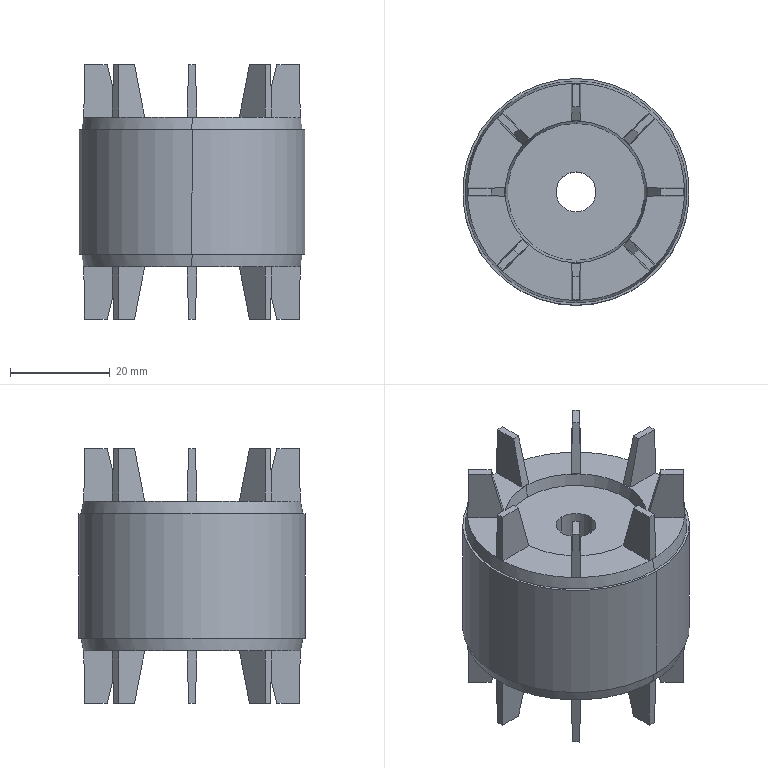Part | STEP file | MSBR-2_1_1_1_1 | 1 solid | 98 faces | box 45.4 x 45.4 x 51 mm | volume 45376 mm3 | plane 86 | cone 8 | cylinder 4 | commonest cylinder face diameters 8 x2 45.4 x2